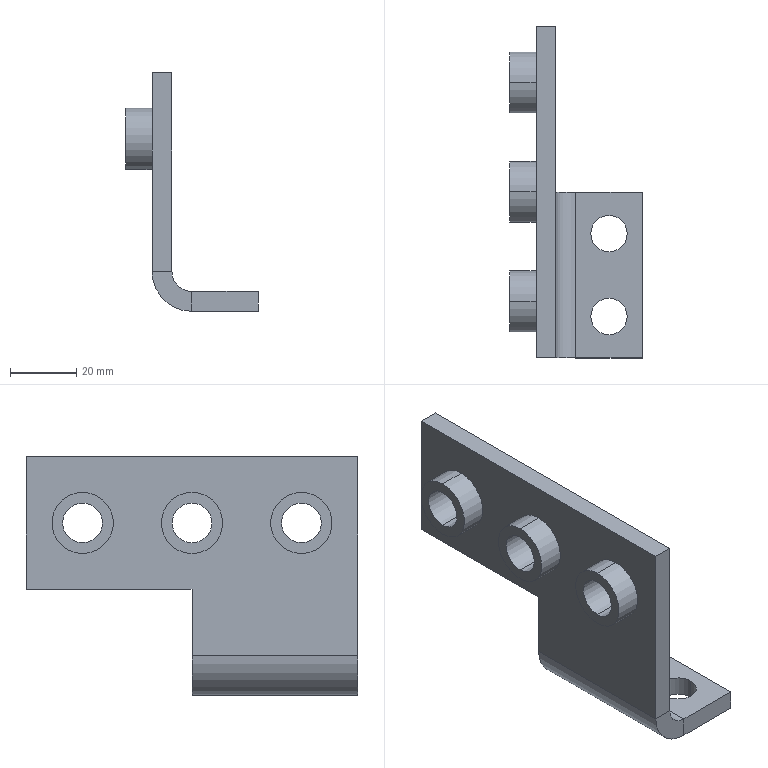Part | STEP file | 64665871 | 1 solid | 35 faces | box 39.9 x 100 x 72 mm | volume 40755 mm3 | cylinder 18 | plane 17 | commonest cylinder face diameters 12 x7 18.5 x6 11 x4 24 x1